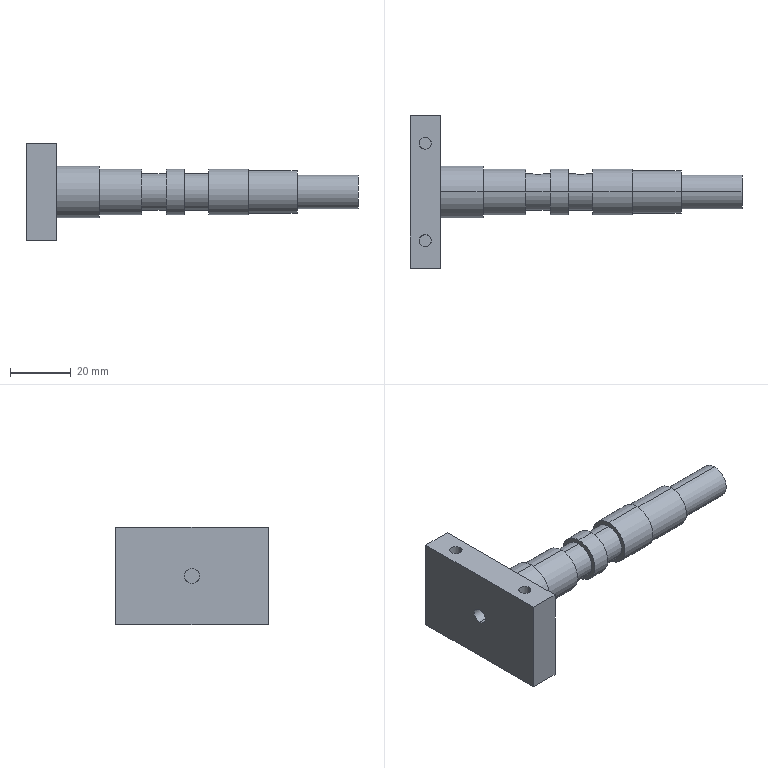Part | SolidWorks | features ICE 7, RevCut 2, Extrusion 1, RefAxis 1 | 1 solid | 56 faces | box 109 x 50 x 32 mm | volume 28769 mm3 | cylinder 38 | plane 18 | commonest cylinder face diameters 4 x20 15 x6 12 x4 5 x2 11 x2 14 x2